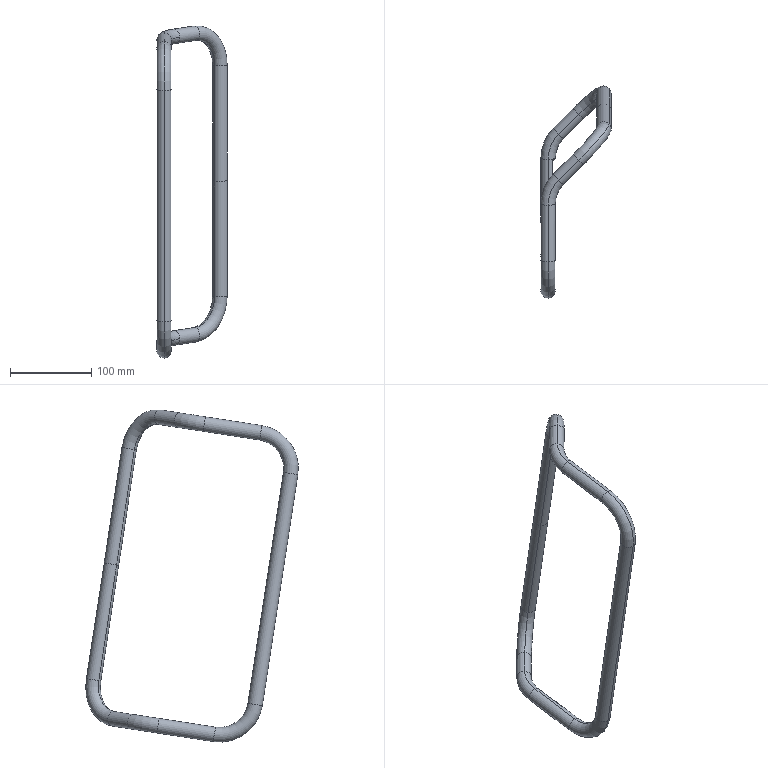Part | SolidWorks | features BaseBody 1 | 1 solid | 112 faces | box 86.742 x 261.941 x 409.573 mm | volume 113336 mm3 | cylinder 50 | torus 28 | plane 28 | cone 4 | spline 2 | commonest cylinder face diameters 9.1 x14 14 x14 18 x14 4 x4 4.1 x2 8 x2